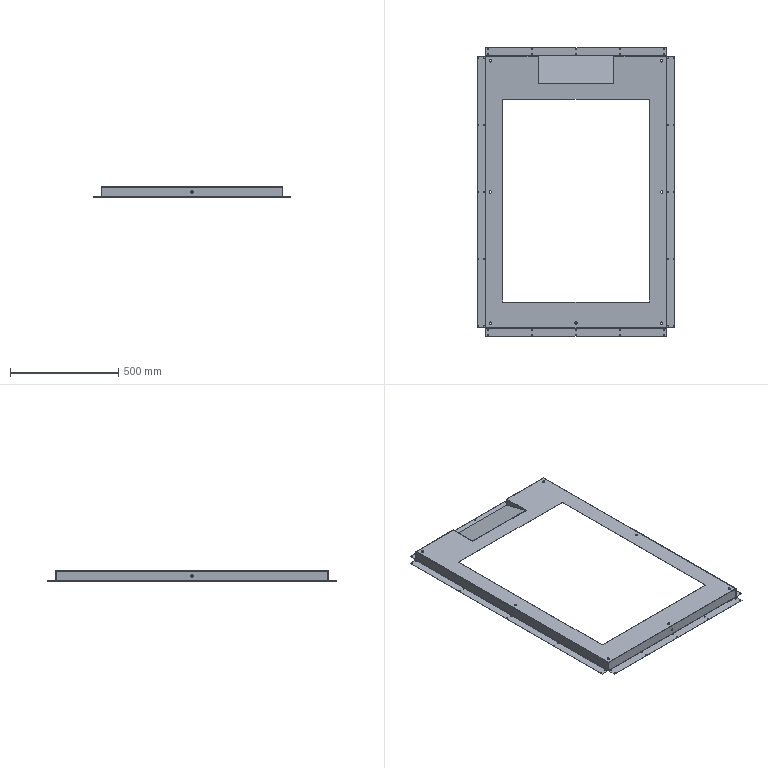Part | SolidWorks | 2 solids | 204 faces | box 913 x 1333 x 48 mm | volume 765196 mm3 | cylinder 122 | plane 70 | spline 12 | commonest cylinder face diameters 4.2 x80 11 x14 0.4 x11 2.4 x11 10 x6